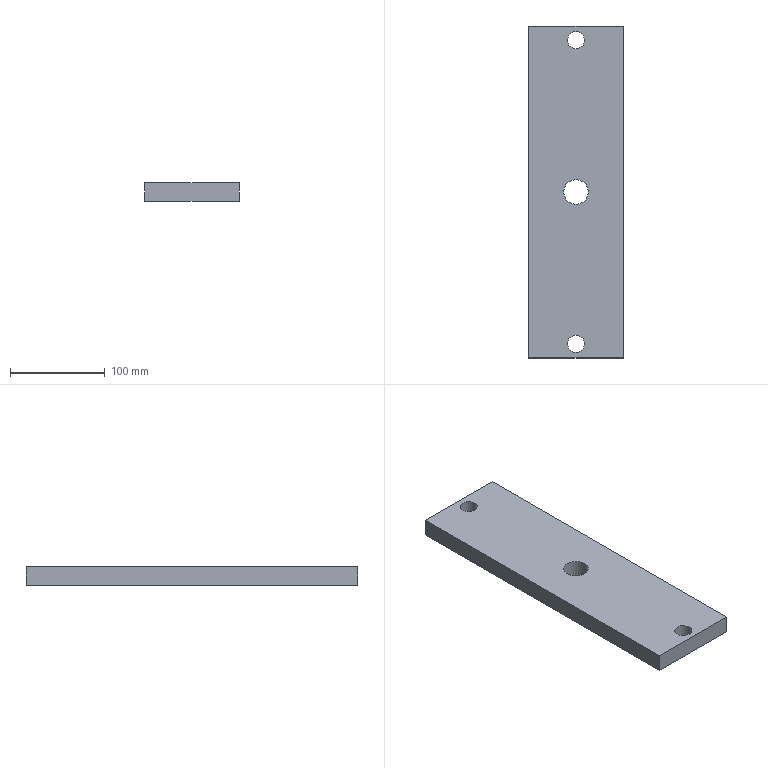Part | NX | features solid 2 | 1 solid | 9 faces | box 100 x 350 x 19 mm | volume 645243 mm3 | plane 6 | cylinder 3 | commonest cylinder face diameters 18 x2 26 x1
STEP:
#1=CARTESIAN_POINT('',(250.,-265.,-186.));
#2=VERTEX_POINT('',#1);
#3=CARTESIAN_POINT('',(150.,-265.,-186.));
#4=VERTEX_POINT('',#3);
#5=CARTESIAN_POINT('',(250.,-265.,-186.));
#6=DIRECTION('',(-1.,0.,0.));
#7=VECTOR('',#6,1000.);
#8=LINE('',#5,#7);
#9=EDGE_CURVE('',#2,#4,#8,.T.);
#10=ORIENTED_EDGE('',*,*,#9,.T.);
#11=CARTESIAN_POINT('',(150.,-265.,-205.));
#12=VERTEX_POINT('',#11);
#13=CARTESIAN_POINT('',(150.,-265.,-205.));
#14=DIRECTION('',(0.,0.,1.));
#15=VECTOR('',#14,1000.);
#16=LINE('',#13,#15);
#17=EDGE_CURVE('',#12,#4,#16,.T.);
#18=ORIENTED_EDGE('',*,*,#17,.F.);
#19=CARTESIAN_POINT('',(250.,-265.,-205.));
#20=VERTEX_POINT('',#19);
#21=CARTESIAN_POINT('',(250.,-265.,-205.));
#22=DIRECTION('',(-1.,0.,0.));
#23=VECTOR('',#22,1000.);
#24=LINE('',#21,#23);
#25=EDGE_CURVE('',#20,#12,#24,.T.);
#26=ORIENTED_EDGE('',*,*,#25,.F.);
#27=CARTESIAN_POINT('',(250.,-265.,-205.));
#28=DIRECTION('',(0.,0.,1.));
#29=VECTOR('',#28,1000.);
#30=LINE('',#27,#29);
#31=EDGE_CURVE('',#20,#2,#30,.T.);
#32=ORIENTED_EDGE('',*,*,#31,.T.);
#33=EDGE_LOOP('',(#10,#18,#26,#32));
#34=FACE_BOUND('',#33,.T.);
#35=CARTESIAN_POINT('',(250.,-265.,-205.));
#36=DIRECTION('',(0.,1.,0.));
#37=DIRECTION('',(0.,0.,1.));
#38=AXIS2_PLACEMENT_3D('',#35,#36,#37);
#39=PLANE('',#38);
#40=ADVANCED_FACE('',(#34),#39,.F.);
#41=CARTESIAN_POINT('',(150.,85.,-186.));
#42=VERTEX_POINT('',#41);
#43=CARTESIAN_POINT('',(150.,-265.,-186.));
#44=DIRECTION('',(0.,1.,0.));
#45=VECTOR('',#44,1000.);
#46=LINE('',#43,#45);
#47=EDGE_CURVE('',#4,#42,#46,.T.);
#48=ORIENTED_EDGE('',*,*,#47,.T.);
#49=CARTESIAN_POINT('',(150.,85.,-205.));
#50=VERTEX_POINT('',#49);
#51=CARTESIAN_POINT('',(150.,85.,-205.));
#52=DIRECTION('',(0.,0.,1.));
#53=VECTOR('',#52,1000.);
#54=LINE('',#51,#53);
#55=EDGE_CURVE('',#50,#42,#54,.T.);
#56=ORIENTED_EDGE('',*,*,#55,.F.);
#57=CARTESIAN_POINT('',(150.,-265.,-205.));
#58=DIRECTION('',(0.,1.,0.));
#59=VECTOR('',#58,1000.);
#60=LINE('',#57,#59);
#61=EDGE_CURVE('',#12,#50,#60,.T.);
#62=ORIENTED_EDGE('',*,*,#61,.F.);
#63=ORIENTED_EDGE('',*,*,#17,.T.);
#64=EDGE_LOOP('',(#48,#56,#62,#63));
#65=FACE_BOUND('',#64,.T.);
#66=CARTESIAN_POINT('',(150.,-265.,-205.));
#67=DIRECTION('',(1.,0.,0.));
#68=DIRECTION('',(0.,1.,0.));
#69=AXIS2_PLACEMENT_3D('',#66,#67,#68);
#70=PLANE('',#69);
#71=ADVANCED_FACE('',(#65),#70,.F.);
#72=CARTESIAN_POINT('',(250.,85.,-186.));
#73=VERTEX_POINT('',#72);
#74=CARTESIAN_POINT('',(150.,85.,-186.));
#75=DIRECTION('',(1.,0.,0.));
#76=VECTOR('',#75,1000.);
#77=LINE('',#74,#76);
#78=EDGE_CURVE('',#42,#73,#77,.T.);
#79=ORIENTED_EDGE('',*,*,#78,.T.);
#80=CARTESIAN_POINT('',(250.,85.,-205.));
#81=VERTEX_POINT('',#80);
#82=CARTESIAN_POINT('',(250.,85.,-205.));
#83=DIRECTION('',(0.,0.,1.));
#84=VECTOR('',#83,1000.);
#85=LINE('',#82,#84);
#86=EDGE_CURVE('',#81,#73,#85,.T.);
#87=ORIENTED_EDGE('',*,*,#86,.F.);
#88=CARTESIAN_POINT('',(150.,85.,-205.));
#89=DIRECTION('',(1.,0.,0.));
#90=VECTOR('',#89,1000.);
#91=LINE('',#88,#90);
#92=EDGE_CURVE('',#50,#81,#91,.T.);
#93=ORIENTED_EDGE('',*,*,#92,.F.);
#94=ORIENTED_EDGE('',*,*,#55,.T.);
#95=EDGE_LOOP('',(#79,#87,#93,#94));
#96=FACE_BOUND('',#95,.T.);
#97=CARTESIAN_POINT('',(150.,85.,-205.));
#98=DIRECTION('',(0.,-1.,0.));
#99=DIRECTION('',(0.,0.,-1.));
#100=AXIS2_PLACEMENT_3D('',#97,#98,#99);
#101=PLANE('',#100);
#102=ADVANCED_FACE('',(#96),#101,.F.);
#103=CARTESIAN_POINT('',(200.,-103.,-205.));
#104=VERTEX_POINT('',#103);
#105=CARTESIAN_POINT('',(200.,-90.,-205.));
#106=DIRECTION('',(0.,0.,1.));
#107=DIRECTION('',(0.,-1.,0.));
#108=AXIS2_PLACEMENT_3D('',#105,#106,#107);
#109=CIRCLE('',#108,13.);
#110=EDGE_CURVE('',#104,#104,#109,.F.);
#111=ORIENTED_EDGE('',*,*,#110,.T.);
#112=EDGE_LOOP('',(#111));
#113=FACE_BOUND('',#112,.T.);
#114=CARTESIAN_POINT('',(200.,-103.,-186.));
#115=VERTEX_POINT('',#114);
#116=CARTESIAN_POINT('',(200.,-90.,-186.));
#117=DIRECTION('',(0.,0.,1.));
#118=DIRECTION('',(0.,-1.,0.));
#119=AXIS2_PLACEMENT_3D('',#116,#117,#118);
#120=CIRCLE('',#119,13.);
#121=EDGE_CURVE('',#115,#115,#120,.F.);
#122=ORIENTED_EDGE('',*,*,#121,.F.);
#123=EDGE_LOOP('',(#122));
#124=FACE_BOUND('',#123,.T.);
#125=CARTESIAN_POINT('',(200.,-90.,-205.));
#126=DIRECTION('',(0.,0.,1.));
#127=DIRECTION('',(0.,-1.,0.));
#128=AXIS2_PLACEMENT_3D('',#125,#126,#127);
#129=CYLINDRICAL_SURFACE('',#128,13.);
#130=ADVANCED_FACE('',(#113,#124),#129,.F.);
#131=CARTESIAN_POINT('',(250.,85.,-186.));
#132=DIRECTION('',(0.,-1.,0.));
#133=VECTOR('',#132,1000.);
#134=LINE('',#131,#133);
#135=EDGE_CURVE('',#73,#2,#134,.T.);
#136=ORIENTED_EDGE('',*,*,#135,.T.);
#137=ORIENTED_EDGE('',*,*,#31,.F.);
#138=CARTESIAN_POINT('',(250.,85.,-205.));
#139=DIRECTION('',(0.,-1.,0.));
#140=VECTOR('',#139,1000.);
#141=LINE('',#138,#140);
#142=EDGE_CURVE('',#81,#20,#141,.T.);
#143=ORIENTED_EDGE('',*,*,#142,.F.);
#144=ORIENTED_EDGE('',*,*,#86,.T.);
#145=EDGE_LOOP('',(#136,#137,#143,#144));
#146=FACE_BOUND('',#145,.T.);
#147=CARTESIAN_POINT('',(250.,85.,-205.));
#148=DIRECTION('',(-1.,0.,0.));
#149=DIRECTION('',(0.,0.,-1.));
#150=AXIS2_PLACEMENT_3D('',#147,#148,#149);
#151=PLANE('',#150);
#152=ADVANCED_FACE('',(#146),#151,.F.);
#153=CARTESIAN_POINT('',(200.,-259.,-205.));
#154=VERTEX_POINT('',#153);
#155=CARTESIAN_POINT('',(200.,-250.,-205.));
#156=DIRECTION('',(0.,0.,-1.));
#157=DIRECTION('',(0.,-1.,0.));
#158=AXIS2_PLACEMENT_3D('',#155,#156,#157);
#159=CIRCLE('',#158,9.);
#160=EDGE_CURVE('',#154,#154,#159,.T.);
#161=ORIENTED_EDGE('',*,*,#160,.T.);
#162=EDGE_LOOP('',(#161));
#163=FACE_BOUND('',#162,.T.);
#164=CARTESIAN_POINT('',(200.,-259.,-186.));
#165=VERTEX_POINT('',#164);
#166=CARTESIAN_POINT('',(200.,-250.,-186.));
#167=DIRECTION('',(0.,0.,-1.));
#168=DIRECTION('',(0.,-1.,0.));
#169=AXIS2_PLACEMENT_3D('',#166,#167,#168);
#170=CIRCLE('',#169,9.);
#171=EDGE_CURVE('',#165,#165,#170,.T.);
#172=ORIENTED_EDGE('',*,*,#171,.F.);
#173=EDGE_LOOP('',(#172));
#174=FACE_BOUND('',#173,.T.);
#175=CARTESIAN_POINT('',(200.,-250.,-205.));
#176=DIRECTION('',(0.,0.,1.));
#177=DIRECTION('',(0.,-1.,0.));
#178=AXIS2_PLACEMENT_3D('',#175,#176,#177);
#179=CYLINDRICAL_SURFACE('',#178,9.);
#180=ADVANCED_FACE('',(#163,#174),#179,.F.);
#181=CARTESIAN_POINT('',(200.,79.,-205.));
#182=VERTEX_POINT('',#181);
#183=CARTESIAN_POINT('',(200.,70.,-205.));
#184=DIRECTION('',(0.,0.,1.));
#185=DIRECTION('',(0.,1.,0.));
#186=AXIS2_PLACEMENT_3D('',#183,#184,#185);
#187=CIRCLE('',#186,9.);
#188=EDGE_CURVE('',#182,#182,#187,.T.);
#189=ORIENTED_EDGE('',*,*,#188,.F.);
#190=EDGE_LOOP('',(#189));
#191=FACE_BOUND('',#190,.T.);
#192=CARTESIAN_POINT('',(200.,79.,-186.));
#193=VERTEX_POINT('',#192);
#194=CARTESIAN_POINT('',(200.,70.,-186.));
#195=DIRECTION('',(0.,0.,1.));
#196=DIRECTION('',(0.,1.,0.));
#197=AXIS2_PLACEMENT_3D('',#194,#195,#196);
#198=CIRCLE('',#197,9.);
#199=EDGE_CURVE('',#193,#193,#198,.T.);
#200=ORIENTED_EDGE('',*,*,#199,.T.);
#201=EDGE_LOOP('',(#200));
#202=FACE_BOUND('',#201,.T.);
#203=CARTESIAN_POINT('',(200.,70.,-205.));
#204=DIRECTION('',(0.,0.,1.));
#205=DIRECTION('',(0.,-1.,0.));
#206=AXIS2_PLACEMENT_3D('',#203,#204,#205);
#207=CYLINDRICAL_SURFACE('',#206,9.);
#208=ADVANCED_FACE('',(#191,#202),#207,.F.);
#209=ORIENTED_EDGE('',*,*,#160,.F.);
#210=EDGE_LOOP('',(#209));
#211=FACE_BOUND('',#210,.T.);
#212=ORIENTED_EDGE('',*,*,#25,.T.);
#213=ORIENTED_EDGE('',*,*,#61,.T.);
#214=ORIENTED_EDGE('',*,*,#92,.T.);
#215=ORIENTED_EDGE('',*,*,#142,.T.);
#216=EDGE_LOOP('',(#212,#213,#214,#215));
#217=FACE_BOUND('',#216,.T.);
#218=ORIENTED_EDGE('',*,*,#110,.F.);
#219=EDGE_LOOP('',(#218));
#220=FACE_BOUND('',#219,.T.);
#221=ORIENTED_EDGE('',*,*,#188,.T.);
#222=EDGE_LOOP('',(#221));
#223=FACE_BOUND('',#222,.T.);
#224=CARTESIAN_POINT('',(250.,-265.,-205.));
#225=DIRECTION('',(0.,0.,1.));
#226=DIRECTION('',(0.,-1.,0.));
#227=AXIS2_PLACEMENT_3D('',#224,#225,#226);
#228=PLANE('',#227);
#229=ADVANCED_FACE('',(#211,#217,#220,#223),#228,.F.);
#230=ORIENTED_EDGE('',*,*,#171,.T.);
#231=EDGE_LOOP('',(#230));
#232=FACE_BOUND('',#231,.T.);
#233=ORIENTED_EDGE('',*,*,#9,.F.);
#234=ORIENTED_EDGE('',*,*,#135,.F.);
#235=ORIENTED_EDGE('',*,*,#78,.F.);
#236=ORIENTED_EDGE('',*,*,#47,.F.);
#237=EDGE_LOOP('',(#233,#234,#235,#236));
#238=FACE_BOUND('',#237,.T.);
#239=ORIENTED_EDGE('',*,*,#121,.T.);
#240=EDGE_LOOP('',(#239));
#241=FACE_BOUND('',#240,.T.);
#242=ORIENTED_EDGE('',*,*,#199,.F.);
#243=EDGE_LOOP('',(#242));
#244=FACE_BOUND('',#243,.T.);
#245=CARTESIAN_POINT('',(250.,-265.,-186.));
#246=DIRECTION('',(0.,0.,1.));
#247=DIRECTION('',(0.,-1.,0.));
#248=AXIS2_PLACEMENT_3D('',#245,#246,#247);
#249=PLANE('',#248);
#250=ADVANCED_FACE('',(#232,#238,#241,#244),#249,.T.);
#251=CLOSED_SHELL('',(#40,#71,#102,#130,#152,#180,#208,#229,#250));
#252=MANIFOLD_SOLID_BREP('',#251);
#253=(LENGTH_UNIT()NAMED_UNIT(*)SI_UNIT(.MILLI.,.METRE.));
#254=UNCERTAINTY_MEASURE_WITH_UNIT(LENGTH_MEASURE(0.00001),#253,'','');
#255=(NAMED_UNIT(*)PLANE_ANGLE_UNIT()SI_UNIT($,.RADIAN.));
#256=(NAMED_UNIT(*)SI_UNIT($,.STERADIAN.)SOLID_ANGLE_UNIT());
#257=(GEOMETRIC_REPRESENTATION_CONTEXT(3)GLOBAL_UNCERTAINTY_ASSIGNED_CONTEXT((#254))GLOBAL_UNIT_ASSIGNED_CONTEXT((#253,#255,#256))REPRESENTATION_CONTEXT('',''));
#258=ADVANCED_BREP_SHAPE_REPRESENTATION('',(#252),#257);